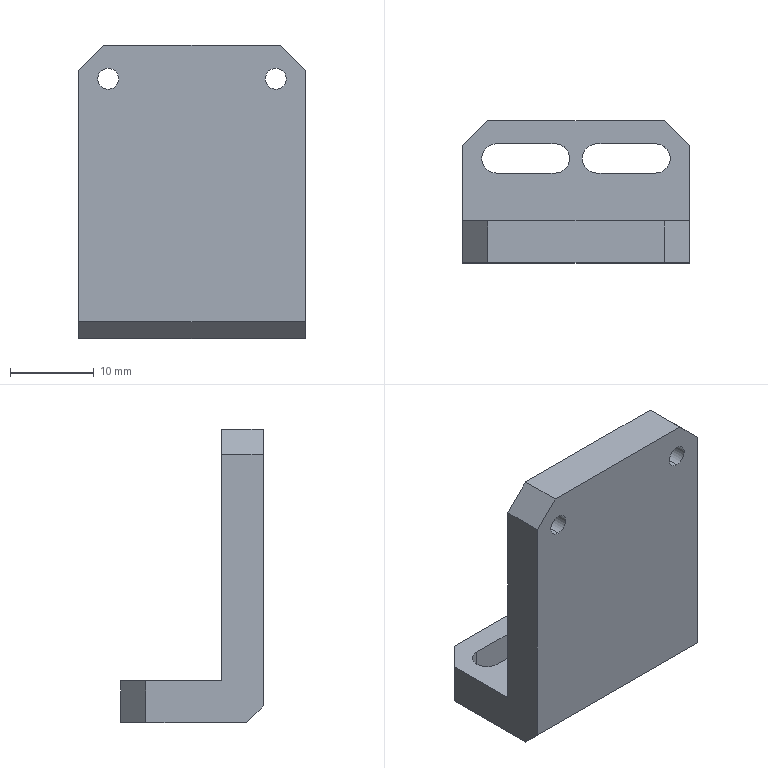Part | NX | features BREP 1 | 1 solid | 27 faces | box 27 x 17 x 35 mm | volume 5811 mm3 | plane 17 | cylinder 10 | commonest cylinder face diameters 3.5 x6 2.5 x4
STEP:
#1=CARTESIAN_POINT('',(-13.5,-3.,-17.5));
#2=VERTEX_POINT('',#1);
#3=CARTESIAN_POINT('',(-13.5,-5.,-15.5));
#4=VERTEX_POINT('',#3);
#5=CARTESIAN_POINT('',(-13.5,-5.,-15.5));
#6=DIRECTION('',(0.,-0.7071,0.7071));
#7=VECTOR('',#6,1000.);
#8=LINE('',#5,#7);
#9=EDGE_CURVE('',#2,#4,#8,.T.);
#10=ORIENTED_EDGE('',*,*,#9,.F.);
#11=CARTESIAN_POINT('',(13.5,-3.,-17.5));
#12=VERTEX_POINT('',#11);
#13=CARTESIAN_POINT('',(0.,-3.,-17.5));
#14=DIRECTION('',(-1.,0.,0.));
#15=VECTOR('',#14,1000.);
#16=LINE('',#13,#15);
#17=EDGE_CURVE('',#12,#2,#16,.T.);
#18=ORIENTED_EDGE('',*,*,#17,.F.);
#19=CARTESIAN_POINT('',(13.5,-5.,-15.5));
#20=VERTEX_POINT('',#19);
#21=CARTESIAN_POINT('',(13.5,-5.,-15.5));
#22=DIRECTION('',(0.,0.7071,-0.7071));
#23=VECTOR('',#22,1000.);
#24=LINE('',#21,#23);
#25=EDGE_CURVE('',#20,#12,#24,.T.);
#26=ORIENTED_EDGE('',*,*,#25,.F.);
#27=CARTESIAN_POINT('',(-13.5,-5.,-15.5));
#28=DIRECTION('',(1.,0.,0.));
#29=VECTOR('',#28,1000.);
#30=LINE('',#27,#29);
#31=EDGE_CURVE('',#4,#20,#30,.T.);
#32=ORIENTED_EDGE('',*,*,#31,.F.);
#33=EDGE_LOOP('',(#10,#18,#26,#32));
#34=FACE_BOUND('',#33,.T.);
#35=CARTESIAN_POINT('',(-13.5,-5.,-15.5));
#36=DIRECTION('',(0.,0.7071,0.7071));
#37=DIRECTION('',(1.,0.,0.));
#38=AXIS2_PLACEMENT_3D('',#35,#36,#37);
#39=PLANE('',#38);
#40=ADVANCED_FACE('',(#34),#39,.F.);
#41=CARTESIAN_POINT('',(-13.5,0.,14.5));
#42=VERTEX_POINT('',#41);
#43=CARTESIAN_POINT('',(-10.5,0.,17.5));
#44=VERTEX_POINT('',#43);
#45=CARTESIAN_POINT('',(-10.5,0.,17.5));
#46=DIRECTION('',(0.7071,0.,0.7071));
#47=VECTOR('',#46,1000.);
#48=LINE('',#45,#47);
#49=EDGE_CURVE('',#42,#44,#48,.T.);
#50=ORIENTED_EDGE('',*,*,#49,.F.);
#51=CARTESIAN_POINT('',(-13.5,-5.,14.5));
#52=VERTEX_POINT('',#51);
#53=CARTESIAN_POINT('',(-13.5,0.,14.5));
#54=DIRECTION('',(0.,1.,0.));
#55=VECTOR('',#54,1000.);
#56=LINE('',#53,#55);
#57=EDGE_CURVE('',#52,#42,#56,.T.);
#58=ORIENTED_EDGE('',*,*,#57,.F.);
#59=CARTESIAN_POINT('',(-10.5,-5.,17.5));
#60=VERTEX_POINT('',#59);
#61=CARTESIAN_POINT('',(-10.5,-5.,17.5));
#62=DIRECTION('',(-0.7071,0.,-0.7071));
#63=VECTOR('',#62,1000.);
#64=LINE('',#61,#63);
#65=EDGE_CURVE('',#60,#52,#64,.T.);
#66=ORIENTED_EDGE('',*,*,#65,.F.);
#67=CARTESIAN_POINT('',(-10.5,-5.,17.5));
#68=DIRECTION('',(0.,-1.,0.));
#69=VECTOR('',#68,1000.);
#70=LINE('',#67,#69);
#71=EDGE_CURVE('',#44,#60,#70,.T.);
#72=ORIENTED_EDGE('',*,*,#71,.F.);
#73=EDGE_LOOP('',(#50,#58,#66,#72));
#74=FACE_BOUND('',#73,.T.);
#75=CARTESIAN_POINT('',(-10.5,0.,17.5));
#76=DIRECTION('',(-0.7071,0.,0.7071));
#77=DIRECTION('',(0.,1.,0.));
#78=AXIS2_PLACEMENT_3D('',#75,#76,#77);
#79=PLANE('',#78);
#80=ADVANCED_FACE('',(#74),#79,.T.);
#81=CARTESIAN_POINT('',(13.5,-5.,14.5));
#82=VERTEX_POINT('',#81);
#83=CARTESIAN_POINT('',(10.5,-5.,17.5));
#84=VERTEX_POINT('',#83);
#85=CARTESIAN_POINT('',(10.5,-5.,17.5));
#86=DIRECTION('',(-0.7071,0.,0.7071));
#87=VECTOR('',#86,1000.);
#88=LINE('',#85,#87);
#89=EDGE_CURVE('',#82,#84,#88,.T.);
#90=ORIENTED_EDGE('',*,*,#89,.F.);
#91=CARTESIAN_POINT('',(13.5,0.,14.5));
#92=VERTEX_POINT('',#91);
#93=CARTESIAN_POINT('',(13.5,-5.,14.5));
#94=DIRECTION('',(0.,-1.,0.));
#95=VECTOR('',#94,1000.);
#96=LINE('',#93,#95);
#97=EDGE_CURVE('',#92,#82,#96,.T.);
#98=ORIENTED_EDGE('',*,*,#97,.F.);
#99=CARTESIAN_POINT('',(10.5,0.,17.5));
#100=VERTEX_POINT('',#99);
#101=CARTESIAN_POINT('',(10.5,0.,17.5));
#102=DIRECTION('',(0.7071,0.,-0.7071));
#103=VECTOR('',#102,1000.);
#104=LINE('',#101,#103);
#105=EDGE_CURVE('',#100,#92,#104,.T.);
#106=ORIENTED_EDGE('',*,*,#105,.F.);
#107=CARTESIAN_POINT('',(10.5,0.,17.5));
#108=DIRECTION('',(0.,1.,0.));
#109=VECTOR('',#108,1000.);
#110=LINE('',#107,#109);
#111=EDGE_CURVE('',#84,#100,#110,.T.);
#112=ORIENTED_EDGE('',*,*,#111,.F.);
#113=EDGE_LOOP('',(#90,#98,#106,#112));
#114=FACE_BOUND('',#113,.T.);
#115=CARTESIAN_POINT('',(10.5,0.,17.5));
#116=DIRECTION('',(0.7071,0.,0.7071));
#117=DIRECTION('',(0.,-1.,0.));
#118=AXIS2_PLACEMENT_3D('',#115,#116,#117);
#119=PLANE('',#118);
#120=ADVANCED_FACE('',(#114),#119,.T.);
#121=CARTESIAN_POINT('',(10.5,12.,-17.5));
#122=VERTEX_POINT('',#121);
#123=CARTESIAN_POINT('',(13.5,9.,-17.5));
#124=VERTEX_POINT('',#123);
#125=CARTESIAN_POINT('',(13.5,9.,-17.5));
#126=DIRECTION('',(0.7071,-0.7071,0.));
#127=VECTOR('',#126,1000.);
#128=LINE('',#125,#127);
#129=EDGE_CURVE('',#122,#124,#128,.T.);
#130=ORIENTED_EDGE('',*,*,#129,.F.);
#131=CARTESIAN_POINT('',(10.5,12.,-12.5));
#132=VERTEX_POINT('',#131);
#133=CARTESIAN_POINT('',(10.5,12.,-17.5));
#134=DIRECTION('',(0.,0.,-1.));
#135=VECTOR('',#134,1000.);
#136=LINE('',#133,#135);
#137=EDGE_CURVE('',#132,#122,#136,.T.);
#138=ORIENTED_EDGE('',*,*,#137,.F.);
#139=CARTESIAN_POINT('',(13.5,9.,-12.5));
#140=VERTEX_POINT('',#139);
#141=CARTESIAN_POINT('',(24.5,-2.,-12.5));
#142=DIRECTION('',(-0.7071,0.7071,0.));
#143=VECTOR('',#142,1000.);
#144=LINE('',#141,#143);
#145=EDGE_CURVE('',#140,#132,#144,.T.);
#146=ORIENTED_EDGE('',*,*,#145,.F.);
#147=CARTESIAN_POINT('',(13.5,9.,-12.5));
#148=DIRECTION('',(0.,0.,1.));
#149=VECTOR('',#148,1000.);
#150=LINE('',#147,#149);
#151=EDGE_CURVE('',#124,#140,#150,.T.);
#152=ORIENTED_EDGE('',*,*,#151,.F.);
#153=EDGE_LOOP('',(#130,#138,#146,#152));
#154=FACE_BOUND('',#153,.T.);
#155=CARTESIAN_POINT('',(13.5,9.,17.5));
#156=DIRECTION('',(0.7071,0.7071,0.));
#157=DIRECTION('',(0.,0.,-1.));
#158=AXIS2_PLACEMENT_3D('',#155,#156,#157);
#159=PLANE('',#158);
#160=ADVANCED_FACE('',(#154),#159,.T.);
#161=CARTESIAN_POINT('',(-10.5,12.,-12.5));
#162=VERTEX_POINT('',#161);
#163=CARTESIAN_POINT('',(-13.5,9.,-12.5));
#164=VERTEX_POINT('',#163);
#165=CARTESIAN_POINT('',(2.,24.5,-12.5));
#166=DIRECTION('',(-0.7071,-0.7071,0.));
#167=VECTOR('',#166,1000.);
#168=LINE('',#165,#167);
#169=EDGE_CURVE('',#162,#164,#168,.T.);
#170=ORIENTED_EDGE('',*,*,#169,.F.);
#171=CARTESIAN_POINT('',(-10.5,12.,-17.5));
#172=VERTEX_POINT('',#171);
#173=CARTESIAN_POINT('',(-10.5,12.,-12.5));
#174=DIRECTION('',(0.,0.,1.));
#175=VECTOR('',#174,1000.);
#176=LINE('',#173,#175);
#177=EDGE_CURVE('',#172,#162,#176,.T.);
#178=ORIENTED_EDGE('',*,*,#177,.F.);
#179=CARTESIAN_POINT('',(-13.5,9.,-17.5));
#180=VERTEX_POINT('',#179);
#181=CARTESIAN_POINT('',(-13.5,9.,-17.5));
#182=DIRECTION('',(0.7071,0.7071,0.));
#183=VECTOR('',#182,1000.);
#184=LINE('',#181,#183);
#185=EDGE_CURVE('',#180,#172,#184,.T.);
#186=ORIENTED_EDGE('',*,*,#185,.F.);
#187=CARTESIAN_POINT('',(-13.5,9.,-17.5));
#188=DIRECTION('',(0.,0.,-1.));
#189=VECTOR('',#188,1000.);
#190=LINE('',#187,#189);
#191=EDGE_CURVE('',#164,#180,#190,.T.);
#192=ORIENTED_EDGE('',*,*,#191,.F.);
#193=EDGE_LOOP('',(#170,#178,#186,#192));
#194=FACE_BOUND('',#193,.T.);
#195=CARTESIAN_POINT('',(-13.5,9.,17.5));
#196=DIRECTION('',(-0.7071,0.7071,0.));
#197=DIRECTION('',(0.,0.,1.));
#198=AXIS2_PLACEMENT_3D('',#195,#196,#197);
#199=PLANE('',#198);
#200=ADVANCED_FACE('',(#194),#199,.T.);
#201=CARTESIAN_POINT('',(9.5,9.25,-12.5));
#202=VERTEX_POINT('',#201);
#203=CARTESIAN_POINT('',(2.5,9.25,-12.5));
#204=VERTEX_POINT('',#203);
#205=CARTESIAN_POINT('',(9.5,9.25,-12.5));
#206=DIRECTION('',(-1.,0.,0.));
#207=VECTOR('',#206,1000.);
#208=LINE('',#205,#207);
#209=EDGE_CURVE('',#202,#204,#208,.T.);
#210=ORIENTED_EDGE('',*,*,#209,.T.);
#211=CARTESIAN_POINT('',(2.5,9.25,-17.5));
#212=VERTEX_POINT('',#211);
#213=CARTESIAN_POINT('',(2.5,9.25,-17.5));
#214=DIRECTION('',(0.,0.,1.));
#215=VECTOR('',#214,1000.);
#216=LINE('',#213,#215);
#217=EDGE_CURVE('',#212,#204,#216,.T.);
#218=ORIENTED_EDGE('',*,*,#217,.F.);
#219=CARTESIAN_POINT('',(9.5,9.25,-17.5));
#220=VERTEX_POINT('',#219);
#221=CARTESIAN_POINT('',(9.5,9.25,-17.5));
#222=DIRECTION('',(-1.,0.,0.));
#223=VECTOR('',#222,1000.);
#224=LINE('',#221,#223);
#225=EDGE_CURVE('',#220,#212,#224,.T.);
#226=ORIENTED_EDGE('',*,*,#225,.F.);
#227=CARTESIAN_POINT('',(9.5,9.25,-17.5));
#228=DIRECTION('',(0.,0.,1.));
#229=VECTOR('',#228,1000.);
#230=LINE('',#227,#229);
#231=EDGE_CURVE('',#220,#202,#230,.T.);
#232=ORIENTED_EDGE('',*,*,#231,.T.);
#233=EDGE_LOOP('',(#210,#218,#226,#232));
#234=FACE_BOUND('',#233,.T.);
#235=CARTESIAN_POINT('',(9.5,9.25,-17.5));
#236=DIRECTION('',(0.,1.,0.));
#237=DIRECTION('',(-1.,0.,0.));
#238=AXIS2_PLACEMENT_3D('',#235,#236,#237);
#239=PLANE('',#238);
#240=ADVANCED_FACE('',(#234),#239,.F.);
#241=CARTESIAN_POINT('',(2.5,5.75,-12.5));
#242=VERTEX_POINT('',#241);
#243=CARTESIAN_POINT('',(2.5,7.5,-12.5));
#244=DIRECTION('',(0.,0.,1.));
#245=DIRECTION('',(1.,0.,0.));
#246=AXIS2_PLACEMENT_3D('',#243,#244,#245);
#247=CIRCLE('',#246,1.75);
#248=EDGE_CURVE('',#204,#242,#247,.T.);
#249=ORIENTED_EDGE('',*,*,#248,.T.);
#250=CARTESIAN_POINT('',(2.5,5.75,-17.5));
#251=VERTEX_POINT('',#250);
#252=CARTESIAN_POINT('',(2.5,5.75,-17.5));
#253=DIRECTION('',(0.,0.,1.));
#254=VECTOR('',#253,1000.);
#255=LINE('',#252,#254);
#256=EDGE_CURVE('',#251,#242,#255,.T.);
#257=ORIENTED_EDGE('',*,*,#256,.F.);
#258=CARTESIAN_POINT('',(2.5,7.5,-17.5));
#259=DIRECTION('',(0.,0.,1.));
#260=DIRECTION('',(1.,0.,0.));
#261=AXIS2_PLACEMENT_3D('',#258,#259,#260);
#262=CIRCLE('',#261,1.75);
#263=EDGE_CURVE('',#212,#251,#262,.T.);
#264=ORIENTED_EDGE('',*,*,#263,.F.);
#265=ORIENTED_EDGE('',*,*,#217,.T.);
#266=EDGE_LOOP('',(#249,#257,#264,#265));
#267=FACE_BOUND('',#266,.T.);
#268=CARTESIAN_POINT('',(2.5,7.5,-17.5));
#269=DIRECTION('',(0.,0.,1.));
#270=DIRECTION('',(1.,0.,0.));
#271=AXIS2_PLACEMENT_3D('',#268,#269,#270);
#272=CYLINDRICAL_SURFACE('',#271,1.75);
#273=ADVANCED_FACE('',(#267),#272,.F.);
#274=CARTESIAN_POINT('',(9.5,5.75,-12.5));
#275=VERTEX_POINT('',#274);
#276=CARTESIAN_POINT('',(9.5,5.75,-12.5));
#277=DIRECTION('',(1.,0.,0.));
#278=VECTOR('',#277,1000.);
#279=LINE('',#276,#278);
#280=EDGE_CURVE('',#242,#275,#279,.T.);
#281=ORIENTED_EDGE('',*,*,#280,.T.);
#282=CARTESIAN_POINT('',(9.5,5.75,-17.5));
#283=VERTEX_POINT('',#282);
#284=CARTESIAN_POINT('',(9.5,5.75,-17.5));
#285=DIRECTION('',(0.,0.,1.));
#286=VECTOR('',#285,1000.);
#287=LINE('',#284,#286);
#288=EDGE_CURVE('',#283,#275,#287,.T.);
#289=ORIENTED_EDGE('',*,*,#288,.F.);
#290=CARTESIAN_POINT('',(9.5,5.75,-17.5));
#291=DIRECTION('',(1.,0.,0.));
#292=VECTOR('',#291,1000.);
#293=LINE('',#290,#292);
#294=EDGE_CURVE('',#251,#283,#293,.T.);
#295=ORIENTED_EDGE('',*,*,#294,.F.);
#296=ORIENTED_EDGE('',*,*,#256,.T.);
#297=EDGE_LOOP('',(#281,#289,#295,#296));
#298=FACE_BOUND('',#297,.T.);
#299=CARTESIAN_POINT('',(9.5,5.75,-17.5));
#300=DIRECTION('',(0.,-1.,0.));
#301=DIRECTION('',(1.,0.,0.));
#302=AXIS2_PLACEMENT_3D('',#299,#300,#301);
#303=PLANE('',#302);
#304=ADVANCED_FACE('',(#298),#303,.F.);
#305=CARTESIAN_POINT('',(11.25,7.5,-17.5));
#306=VERTEX_POINT('',#305);
#307=CARTESIAN_POINT('',(11.25,7.5,-12.5));
#308=VERTEX_POINT('',#307);
#309=CARTESIAN_POINT('',(11.25,7.5,-17.5));
#310=DIRECTION('',(0.,0.,1.));
#311=VECTOR('',#310,1000.);
#312=LINE('',#309,#311);
#313=EDGE_CURVE('',#306,#308,#312,.T.);
#314=ORIENTED_EDGE('',*,*,#313,.F.);
#315=CARTESIAN_POINT('',(9.5,7.5,-17.5));
#316=DIRECTION('',(0.,0.,1.));
#317=DIRECTION('',(1.,0.,0.));
#318=AXIS2_PLACEMENT_3D('',#315,#316,#317);
#319=CIRCLE('',#318,1.75);
#320=EDGE_CURVE('',#283,#306,#319,.T.);
#321=ORIENTED_EDGE('',*,*,#320,.F.);
#322=ORIENTED_EDGE('',*,*,#288,.T.);
#323=CARTESIAN_POINT('',(9.5,7.5,-12.5));
#324=DIRECTION('',(0.,0.,1.));
#325=DIRECTION('',(1.,0.,0.));
#326=AXIS2_PLACEMENT_3D('',#323,#324,#325);
#327=CIRCLE('',#326,1.75);
#328=EDGE_CURVE('',#275,#308,#327,.T.);
#329=ORIENTED_EDGE('',*,*,#328,.T.);
#330=EDGE_LOOP('',(#314,#321,#322,#329));
#331=FACE_BOUND('',#330,.T.);
#332=CARTESIAN_POINT('',(9.5,7.5,-17.5));
#333=DIRECTION('',(0.,0.,1.));
#334=DIRECTION('',(1.,0.,0.));
#335=AXIS2_PLACEMENT_3D('',#332,#333,#334);
#336=CYLINDRICAL_SURFACE('',#335,1.75);
#337=ADVANCED_FACE('',(#331),#336,.F.);
#338=CARTESIAN_POINT('',(-9.5,5.75,-12.5));
#339=VERTEX_POINT('',#338);
#340=CARTESIAN_POINT('',(-2.5,5.75,-12.5));
#341=VERTEX_POINT('',#340);
#342=CARTESIAN_POINT('',(-9.5,5.75,-12.5));
#343=DIRECTION('',(1.,0.,0.));
#344=VECTOR('',#343,1000.);
#345=LINE('',#342,#344);
#346=EDGE_CURVE('',#339,#341,#345,.T.);
#347=ORIENTED_EDGE('',*,*,#346,.T.);
#348=CARTESIAN_POINT('',(-2.5,5.75,-17.5));
#349=VERTEX_POINT('',#348);
#350=CARTESIAN_POINT('',(-2.5,5.75,-17.5));
#351=DIRECTION('',(0.,0.,1.));
#352=VECTOR('',#351,1000.);
#353=LINE('',#350,#352);
#354=EDGE_CURVE('',#349,#341,#353,.T.);
#355=ORIENTED_EDGE('',*,*,#354,.F.);
#356=CARTESIAN_POINT('',(-9.5,5.75,-17.5));
#357=VERTEX_POINT('',#356);
#358=CARTESIAN_POINT('',(-9.5,5.75,-17.5));
#359=DIRECTION('',(1.,0.,0.));
#360=VECTOR('',#359,1000.);
#361=LINE('',#358,#360);
#362=EDGE_CURVE('',#357,#349,#361,.T.);
#363=ORIENTED_EDGE('',*,*,#362,.F.);
#364=CARTESIAN_POINT('',(-9.5,5.75,-17.5));
#365=DIRECTION('',(0.,0.,1.));
#366=VECTOR('',#365,1000.);
#367=LINE('',#364,#366);
#368=EDGE_CURVE('',#357,#339,#367,.T.);
#369=ORIENTED_EDGE('',*,*,#368,.T.);
#370=EDGE_LOOP('',(#347,#355,#363,#369));
#371=FACE_BOUND('',#370,.T.);
#372=CARTESIAN_POINT('',(-9.5,5.75,-17.5));
#373=DIRECTION('',(0.,-1.,0.));
#374=DIRECTION('',(1.,0.,0.));
#375=AXIS2_PLACEMENT_3D('',#372,#373,#374);
#376=PLANE('',#375);
#377=ADVANCED_FACE('',(#371),#376,.F.);
#378=CARTESIAN_POINT('',(-0.75,7.5,-17.5));
#379=VERTEX_POINT('',#378);
#380=CARTESIAN_POINT('',(-0.75,7.5,-12.5));
#381=VERTEX_POINT('',#380);
#382=CARTESIAN_POINT('',(-0.75,7.5,-17.5));
#383=DIRECTION('',(0.,0.,1.));
#384=VECTOR('',#383,1000.);
#385=LINE('',#382,#384);
#386=EDGE_CURVE('',#379,#381,#385,.T.);
#387=ORIENTED_EDGE('',*,*,#386,.F.);
#388=CARTESIAN_POINT('',(-2.5,7.5,-17.5));
#389=DIRECTION('',(0.,0.,1.));
#390=DIRECTION('',(1.,0.,0.));
#391=AXIS2_PLACEMENT_3D('',#388,#389,#390);
#392=CIRCLE('',#391,1.75);
#393=EDGE_CURVE('',#349,#379,#392,.T.);
#394=ORIENTED_EDGE('',*,*,#393,.F.);
#395=ORIENTED_EDGE('',*,*,#354,.T.);
#396=CARTESIAN_POINT('',(-2.5,7.5,-12.5));
#397=DIRECTION('',(0.,0.,1.));
#398=DIRECTION('',(1.,0.,0.));
#399=AXIS2_PLACEMENT_3D('',#396,#397,#398);
#400=CIRCLE('',#399,1.75);
#401=EDGE_CURVE('',#341,#381,#400,.T.);
#402=ORIENTED_EDGE('',*,*,#401,.T.);
#403=EDGE_LOOP('',(#387,#394,#395,#402));
#404=FACE_BOUND('',#403,.T.);
#405=CARTESIAN_POINT('',(-2.5,7.5,-17.5));
#406=DIRECTION('',(0.,0.,1.));
#407=DIRECTION('',(1.,0.,0.));
#408=AXIS2_PLACEMENT_3D('',#405,#406,#407);
#409=CYLINDRICAL_SURFACE('',#408,1.75);
#410=ADVANCED_FACE('',(#404),#409,.F.);
#411=CARTESIAN_POINT('',(-2.5,9.25,-12.5));
#412=VERTEX_POINT('',#411);
#413=CARTESIAN_POINT('',(-9.5,9.25,-12.5));
#414=VERTEX_POINT('',#413);
#415=CARTESIAN_POINT('',(-9.5,9.25,-12.5));
#416=DIRECTION('',(-1.,0.,0.));
#417=VECTOR('',#416,1000.);
#418=LINE('',#415,#417);
#419=EDGE_CURVE('',#412,#414,#418,.T.);
#420=ORIENTED_EDGE('',*,*,#419,.T.);
#421=CARTESIAN_POINT('',(-9.5,9.25,-17.5));
#422=VERTEX_POINT('',#421);
#423=CARTESIAN_POINT('',(-9.5,9.25,-17.5));
#424=DIRECTION('',(0.,0.,1.));
#425=VECTOR('',#424,1000.);
#426=LINE('',#423,#425);
#427=EDGE_CURVE('',#422,#414,#426,.T.);
#428=ORIENTED_EDGE('',*,*,#427,.F.);
#429=CARTESIAN_POINT('',(-2.5,9.25,-17.5));
#430=VERTEX_POINT('',#429);
#431=CARTESIAN_POINT('',(-9.5,9.25,-17.5));
#432=DIRECTION('',(-1.,0.,0.));
#433=VECTOR('',#432,1000.);
#434=LINE('',#431,#433);
#435=EDGE_CURVE('',#430,#422,#434,.T.);
#436=ORIENTED_EDGE('',*,*,#435,.F.);
#437=CARTESIAN_POINT('',(-2.5,9.25,-17.5));
#438=DIRECTION('',(0.,0.,1.));
#439=VECTOR('',#438,1000.);
#440=LINE('',#437,#439);
#441=EDGE_CURVE('',#430,#412,#440,.T.);
#442=ORIENTED_EDGE('',*,*,#441,.T.);
#443=EDGE_LOOP('',(#420,#428,#436,#442));
#444=FACE_BOUND('',#443,.T.);
#445=CARTESIAN_POINT('',(-9.5,9.25,-17.5));
#446=DIRECTION('',(0.,1.,0.));
#447=DIRECTION('',(-1.,0.,0.));
#448=AXIS2_PLACEMENT_3D('',#445,#446,#447);
#449=PLANE('',#448);
#450=ADVANCED_FACE('',(#444),#449,.F.);
#451=CARTESIAN_POINT('',(-9.5,7.5,-12.5));
#452=DIRECTION('',(0.,0.,1.));
#453=DIRECTION('',(1.,0.,0.));
#454=AXIS2_PLACEMENT_3D('',#451,#452,#453);
#455=CIRCLE('',#454,1.75);
#456=EDGE_CURVE('',#414,#339,#455,.T.);
#457=ORIENTED_EDGE('',*,*,#456,.T.);
#458=ORIENTED_EDGE('',*,*,#368,.F.);
#459=CARTESIAN_POINT('',(-9.5,7.5,-17.5));
#460=DIRECTION('',(0.,0.,1.));
#461=DIRECTION('',(1.,0.,0.));
#462=AXIS2_PLACEMENT_3D('',#459,#460,#461);
#463=CIRCLE('',#462,1.75);
#464=EDGE_CURVE('',#422,#357,#463,.T.);
#465=ORIENTED_EDGE('',*,*,#464,.F.);
#466=ORIENTED_EDGE('',*,*,#427,.T.);
#467=EDGE_LOOP('',(#457,#458,#465,#466));
#468=FACE_BOUND('',#467,.T.);
#469=CARTESIAN_POINT('',(-9.5,7.5,-17.5));
#470=DIRECTION('',(0.,0.,1.));
#471=DIRECTION('',(1.,0.,0.));
#472=AXIS2_PLACEMENT_3D('',#469,#470,#471);
#473=CYLINDRICAL_SURFACE('',#472,1.75);
#474=ADVANCED_FACE('',(#468),#473,.F.);
#475=CARTESIAN_POINT('',(26.5,12.,-12.5));
#476=DIRECTION('',(-1.,0.,0.));
#477=VECTOR('',#476,1000.);
#478=LINE('',#475,#477);
#479=EDGE_CURVE('',#132,#162,#478,.T.);
#480=ORIENTED_EDGE('',*,*,#479,.T.);
#481=ORIENTED_EDGE('',*,*,#169,.T.);
#482=CARTESIAN_POINT('',(-13.5,0.,-12.5));
#483=VERTEX_POINT('',#482);
#484=CARTESIAN_POINT('',(-13.5,0.,-12.5));
#485=DIRECTION('',(0.,1.,0.));
#486=VECTOR('',#485,1000.);
#487=LINE('',#484,#486);
#488=EDGE_CURVE('',#483,#164,#487,.T.);
#489=ORIENTED_EDGE('',*,*,#488,.F.);
#490=CARTESIAN_POINT('',(13.5,0.,-12.5));
#491=VERTEX_POINT('',#490);
#492=CARTESIAN_POINT('',(26.5,0.,-12.5));
#493=DIRECTION('',(-1.,0.,0.));
#494=VECTOR('',#493,1000.);
#495=LINE('',#492,#494);
#496=EDGE_CURVE('',#491,#483,#495,.T.);
#497=ORIENTED_EDGE('',*,*,#496,.F.);
#498=CARTESIAN_POINT('',(13.5,0.,-12.5));
#499=DIRECTION('',(0.,-1.,0.));
#500=VECTOR('',#499,1000.);
#501=LINE('',#498,#500);
#502=EDGE_CURVE('',#140,#491,#501,.T.);
#503=ORIENTED_EDGE('',*,*,#502,.F.);
#504=ORIENTED_EDGE('',*,*,#145,.T.);
#505=EDGE_LOOP('',(#480,#481,#489,#497,#503,#504));
#506=FACE_BOUND('',#505,.T.);
#507=ORIENTED_EDGE('',*,*,#456,.F.);
#508=ORIENTED_EDGE('',*,*,#419,.F.);
#509=CARTESIAN_POINT('',(-2.5,7.5,-12.5));
#510=DIRECTION('',(0.,0.,1.));
#511=DIRECTION('',(1.,0.,0.));
#512=AXIS2_PLACEMENT_3D('',#509,#510,#511);
#513=CIRCLE('',#512,1.75);
#514=EDGE_CURVE('',#381,#412,#513,.T.);
#515=ORIENTED_EDGE('',*,*,#514,.F.);
#516=ORIENTED_EDGE('',*,*,#401,.F.);
#517=ORIENTED_EDGE('',*,*,#346,.F.);
#518=EDGE_LOOP('',(#507,#508,#515,#516,#517));
#519=FACE_BOUND('',#518,.T.);
#520=ORIENTED_EDGE('',*,*,#328,.F.);
#521=ORIENTED_EDGE('',*,*,#280,.F.);
#522=ORIENTED_EDGE('',*,*,#248,.F.);
#523=ORIENTED_EDGE('',*,*,#209,.F.);
#524=CARTESIAN_POINT('',(9.5,7.5,-12.5));
#525=DIRECTION('',(0.,0.,1.));
#526=DIRECTION('',(1.,0.,0.));
#527=AXIS2_PLACEMENT_3D('',#524,#525,#526);
#528=CIRCLE('',#527,1.75);
#529=EDGE_CURVE('',#308,#202,#528,.T.);
#530=ORIENTED_EDGE('',*,*,#529,.F.);
#531=EDGE_LOOP('',(#520,#521,#522,#523,#530));
#532=FACE_BOUND('',#531,.T.);
#533=CARTESIAN_POINT('',(26.5,0.,-12.5));
#534=DIRECTION('',(0.,0.,1.));
#535=DIRECTION('',(1.,0.,0.));
#536=AXIS2_PLACEMENT_3D('',#533,#534,#535);
#537=PLANE('',#536);
#538=ADVANCED_FACE('',(#506,#519,#532),#537,.T.);
#539=CARTESIAN_POINT('',(26.5,12.,-17.5));
#540=DIRECTION('',(-1.,0.,0.));
#541=VECTOR('',#540,1000.);
#542=LINE('',#539,#541);
#543=EDGE_CURVE('',#122,#172,#542,.T.);
#544=ORIENTED_EDGE('',*,*,#543,.T.);
#545=ORIENTED_EDGE('',*,*,#177,.T.);
#546=ORIENTED_EDGE('',*,*,#479,.F.);
#547=ORIENTED_EDGE('',*,*,#137,.T.);
#548=EDGE_LOOP('',(#544,#545,#546,#547));
#549=FACE_BOUND('',#548,.T.);
#550=CARTESIAN_POINT('',(26.5,12.,-17.5));
#551=DIRECTION('',(0.,1.,0.));
#552=DIRECTION('',(0.,0.,1.));
#553=AXIS2_PLACEMENT_3D('',#550,#551,#552);
#554=PLANE('',#553);
#555=ADVANCED_FACE('',(#549),#554,.T.);
#556=CARTESIAN_POINT('',(-10.,0.,12.25));
#557=VERTEX_POINT('',#556);
#558=CARTESIAN_POINT('',(-10.,-5.,12.25));
#559=VERTEX_POINT('',#558);
#560=CARTESIAN_POINT('',(-10.,0.,12.25));
#561=DIRECTION('',(0.,1.,0.));
#562=VECTOR('',#561,1000.);
#563=LINE('',#560,#562);
#564=EDGE_CURVE('',#557,#559,#563,.F.);
#565=ORIENTED_EDGE('',*,*,#564,.T.);
#566=CARTESIAN_POINT('',(-10.,-5.,14.75));
#567=VERTEX_POINT('',#566);
#568=CARTESIAN_POINT('',(-10.,-5.,13.5));
#569=DIRECTION('',(0.,1.,0.));
#570=DIRECTION('',(0.,0.,1.));
#571=AXIS2_PLACEMENT_3D('',#568,#569,#570);
#572=CIRCLE('',#571,1.25);
#573=EDGE_CURVE('',#567,#559,#572,.T.);
#574=ORIENTED_EDGE('',*,*,#573,.F.);
#575=CARTESIAN_POINT('',(-10.,0.,14.75));
#576=VERTEX_POINT('',#575);
#577=CARTESIAN_POINT('',(-10.,0.,14.75));
#578=DIRECTION('',(0.,1.,0.));
#579=VECTOR('',#578,1000.);
#580=LINE('',#577,#579);
#581=EDGE_CURVE('',#576,#567,#580,.F.);
#582=ORIENTED_EDGE('',*,*,#581,.F.);
#583=CARTESIAN_POINT('',(-10.,0.,13.5));
#584=DIRECTION('',(0.,1.,0.));
#585=DIRECTION('',(0.,0.,1.));
#586=AXIS2_PLACEMENT_3D('',#583,#584,#585);
#587=CIRCLE('',#586,1.25);
#588=EDGE_CURVE('',#576,#557,#587,.T.);
#589=ORIENTED_EDGE('',*,*,#588,.T.);
#590=EDGE_LOOP('',(#565,#574,#582,#589));
#591=FACE_BOUND('',#590,.T.);
#592=CARTESIAN_POINT('',(-10.,0.,13.5));
#593=DIRECTION('',(0.,1.,0.));
#594=DIRECTION('',(0.,0.,1.));
#595=AXIS2_PLACEMENT_3D('',#592,#593,#594);
#596=CYLINDRICAL_SURFACE('',#595,1.25);
#597=ADVANCED_FACE('',(#591),#596,.F.);
#598=CARTESIAN_POINT('',(10.,0.,12.25));
#599=VERTEX_POINT('',#598);
#600=CARTESIAN_POINT('',(10.,-5.,12.25));
#601=VERTEX_POINT('',#600);
#602=CARTESIAN_POINT('',(10.,0.,12.25));
#603=DIRECTION('',(0.,1.,0.));
#604=VECTOR('',#603,1000.);
#605=LINE('',#602,#604);
#606=EDGE_CURVE('',#599,#601,#605,.F.);
#607=ORIENTED_EDGE('',*,*,#606,.T.);
#608=CARTESIAN_POINT('',(10.,-5.,14.75));
#609=VERTEX_POINT('',#608);
#610=CARTESIAN_POINT('',(10.,-5.,13.5));
#611=DIRECTION('',(0.,1.,0.));
#612=DIRECTION('',(0.,0.,1.));
#613=AXIS2_PLACEMENT_3D('',#610,#611,#612);
#614=CIRCLE('',#613,1.25);
#615=EDGE_CURVE('',#609,#601,#614,.T.);
#616=ORIENTED_EDGE('',*,*,#615,.F.);
#617=CARTESIAN_POINT('',(10.,0.,14.75));
#618=VERTEX_POINT('',#617);
#619=CARTESIAN_POINT('',(10.,0.,14.75));
#620=DIRECTION('',(0.,1.,0.));
#621=VECTOR('',#620,1000.);
#622=LINE('',#619,#621);
#623=EDGE_CURVE('',#618,#609,#622,.F.);
#624=ORIENTED_EDGE('',*,*,#623,.F.);
#625=CARTESIAN_POINT('',(10.,0.,13.5));
#626=DIRECTION('',(0.,1.,0.));
#627=DIRECTION('',(0.,0.,1.));
#628=AXIS2_PLACEMENT_3D('',#625,#626,#627);
#629=CIRCLE('',#628,1.25);
#630=EDGE_CURVE('',#618,#599,#629,.T.);
#631=ORIENTED_EDGE('',*,*,#630,.T.);
#632=EDGE_LOOP('',(#607,#616,#624,#631));
#633=FACE_BOUND('',#632,.T.);
#634=CARTESIAN_POINT('',(10.,0.,13.5));
#635=DIRECTION('',(0.,1.,0.));
#636=DIRECTION('',(0.,0.,1.));
#637=AXIS2_PLACEMENT_3D('',#634,#635,#636);
#638=CYLINDRICAL_SURFACE('',#637,1.25);
#639=ADVANCED_FACE('',(#633),#638,.F.);
#640=CARTESIAN_POINT('',(13.5,-5.,-17.5));
#641=DIRECTION('',(0.,1.,0.));
#642=VECTOR('',#641,1000.);
#643=LINE('',#640,#642);
#644=EDGE_CURVE('',#12,#124,#643,.T.);
#645=ORIENTED_EDGE('',*,*,#644,.F.);
#646=ORIENTED_EDGE('',*,*,#17,.T.);
#647=CARTESIAN_POINT('',(-13.5,0.,-17.5));
#648=DIRECTION('',(0.,-1.,0.));
#649=VECTOR('',#648,1000.);
#650=LINE('',#647,#649);
#651=EDGE_CURVE('',#180,#2,#650,.T.);
#652=ORIENTED_EDGE('',*,*,#651,.F.);
#653=ORIENTED_EDGE('',*,*,#185,.T.);
#654=ORIENTED_EDGE('',*,*,#543,.F.);
#655=ORIENTED_EDGE('',*,*,#129,.T.);
#656=EDGE_LOOP('',(#645,#646,#652,#653,#654,#655));
#657=FACE_BOUND('',#656,.T.);
#658=ORIENTED_EDGE('',*,*,#435,.T.);
#659=ORIENTED_EDGE('',*,*,#464,.T.);
#660=ORIENTED_EDGE('',*,*,#362,.T.);
#661=ORIENTED_EDGE('',*,*,#393,.T.);
#662=CARTESIAN_POINT('',(-2.5,7.5,-17.5));
#663=DIRECTION('',(0.,0.,1.));
#664=DIRECTION('',(1.,0.,0.));
#665=AXIS2_PLACEMENT_3D('',#662,#663,#664);
#666=CIRCLE('',#665,1.75);
#667=EDGE_CURVE('',#379,#430,#666,.T.);
#668=ORIENTED_EDGE('',*,*,#667,.T.);
#669=EDGE_LOOP('',(#658,#659,#660,#661,#668));
#670=FACE_BOUND('',#669,.T.);
#671=ORIENTED_EDGE('',*,*,#294,.T.);
#672=ORIENTED_EDGE('',*,*,#320,.T.);
#673=CARTESIAN_POINT('',(9.5,7.5,-17.5));
#674=DIRECTION('',(0.,0.,1.));
#675=DIRECTION('',(1.,0.,0.));
#676=AXIS2_PLACEMENT_3D('',#673,#674,#675);
#677=CIRCLE('',#676,1.75);
#678=EDGE_CURVE('',#306,#220,#677,.T.);
#679=ORIENTED_EDGE('',*,*,#678,.T.);
#680=ORIENTED_EDGE('',*,*,#225,.T.);
#681=ORIENTED_EDGE('',*,*,#263,.T.);
#682=EDGE_LOOP('',(#671,#672,#679,#680,#681));
#683=FACE_BOUND('',#682,.T.);
#684=CARTESIAN_POINT('',(0.,0.,-17.5));
#685=DIRECTION('',(0.,0.,1.));
#686=DIRECTION('',(1.,0.,0.));
#687=AXIS2_PLACEMENT_3D('',#684,#685,#686);
#688=PLANE('',#687);
#689=ADVANCED_FACE('',(#657,#670,#683),#688,.F.);
#690=CARTESIAN_POINT('',(-13.5,-5.,17.5));
#691=DIRECTION('',(1.,0.,0.));
#692=VECTOR('',#691,1000.);
#693=LINE('',#690,#692);
#694=EDGE_CURVE('',#60,#84,#693,.T.);
#695=ORIENTED_EDGE('',*,*,#694,.T.);
#696=ORIENTED_EDGE('',*,*,#111,.T.);
#697=CARTESIAN_POINT('',(13.5,0.,17.5));
#698=DIRECTION('',(-1.,0.,0.));
#699=VECTOR('',#698,1000.);
#700=LINE('',#697,#699);
#701=EDGE_CURVE('',#100,#44,#700,.T.);
#702=ORIENTED_EDGE('',*,*,#701,.T.);
#703=ORIENTED_EDGE('',*,*,#71,.T.);
#704=EDGE_LOOP('',(#695,#696,#702,#703));
#705=FACE_BOUND('',#704,.T.);
#706=CARTESIAN_POINT('',(0.,0.,17.5));
#707=DIRECTION('',(0.,0.,1.));
#708=DIRECTION('',(1.,0.,0.));
#709=AXIS2_PLACEMENT_3D('',#706,#707,#708);
#710=PLANE('',#709);
#711=ADVANCED_FACE('',(#705),#710,.T.);
#712=CARTESIAN_POINT('',(13.5,-5.,17.5));
#713=DIRECTION('',(0.,0.,-1.));
#714=VECTOR('',#713,1000.);
#715=LINE('',#712,#714);
#716=EDGE_CURVE('',#82,#20,#715,.T.);
#717=ORIENTED_EDGE('',*,*,#716,.T.);
#718=ORIENTED_EDGE('',*,*,#25,.T.);
#719=ORIENTED_EDGE('',*,*,#644,.T.);
#720=ORIENTED_EDGE('',*,*,#151,.T.);
#721=ORIENTED_EDGE('',*,*,#502,.T.);
#722=CARTESIAN_POINT('',(13.5,0.,17.5));
#723=DIRECTION('',(0.,0.,-1.));
#724=VECTOR('',#723,1000.);
#725=LINE('',#722,#724);
#726=EDGE_CURVE('',#92,#491,#725,.T.);
#727=ORIENTED_EDGE('',*,*,#726,.F.);
#728=ORIENTED_EDGE('',*,*,#97,.T.);
#729=EDGE_LOOP('',(#717,#718,#719,#720,#721,#727,#728));
#730=FACE_BOUND('',#729,.T.);
#731=CARTESIAN_POINT('',(13.5,-5.,17.5));
#732=DIRECTION('',(-1.,0.,0.));
#733=DIRECTION('',(0.,0.,1.));
#734=AXIS2_PLACEMENT_3D('',#731,#732,#733);
#735=PLANE('',#734);
#736=ADVANCED_FACE('',(#730),#735,.F.);
#737=CARTESIAN_POINT('',(-13.5,-5.,17.5));
#738=DIRECTION('',(0.,0.,-1.));
#739=VECTOR('',#738,1000.);
#740=LINE('',#737,#739);
#741=EDGE_CURVE('',#52,#4,#740,.T.);
#742=ORIENTED_EDGE('',*,*,#741,.T.);
#743=ORIENTED_EDGE('',*,*,#31,.T.);
#744=ORIENTED_EDGE('',*,*,#716,.F.);
#745=ORIENTED_EDGE('',*,*,#89,.T.);
#746=ORIENTED_EDGE('',*,*,#694,.F.);
#747=ORIENTED_EDGE('',*,*,#65,.T.);
#748=EDGE_LOOP('',(#742,#743,#744,#745,#746,#747));
#749=FACE_BOUND('',#748,.T.);
#750=ORIENTED_EDGE('',*,*,#615,.T.);
#751=CARTESIAN_POINT('',(10.,-5.,13.5));
#752=DIRECTION('',(0.,1.,0.));
#753=DIRECTION('',(0.,0.,1.));
#754=AXIS2_PLACEMENT_3D('',#751,#752,#753);
#755=CIRCLE('',#754,1.25);
#756=EDGE_CURVE('',#601,#609,#755,.T.);
#757=ORIENTED_EDGE('',*,*,#756,.T.);
#758=EDGE_LOOP('',(#750,#757));
#759=FACE_BOUND('',#758,.T.);
#760=ORIENTED_EDGE('',*,*,#573,.T.);
#761=CARTESIAN_POINT('',(-10.,-5.,13.5));
#762=DIRECTION('',(0.,1.,0.));
#763=DIRECTION('',(0.,0.,1.));
#764=AXIS2_PLACEMENT_3D('',#761,#762,#763);
#765=CIRCLE('',#764,1.25);
#766=EDGE_CURVE('',#559,#567,#765,.T.);
#767=ORIENTED_EDGE('',*,*,#766,.T.);
#768=EDGE_LOOP('',(#760,#767));
#769=FACE_BOUND('',#768,.T.);
#770=CARTESIAN_POINT('',(-13.5,-5.,17.5));
#771=DIRECTION('',(0.,1.,0.));
#772=DIRECTION('',(0.,0.,1.));
#773=AXIS2_PLACEMENT_3D('',#770,#771,#772);
#774=PLANE('',#773);
#775=ADVANCED_FACE('',(#749,#759,#769),#774,.F.);
#776=ORIENTED_EDGE('',*,*,#651,.T.);
#777=ORIENTED_EDGE('',*,*,#9,.T.);
#778=ORIENTED_EDGE('',*,*,#741,.F.);
#779=ORIENTED_EDGE('',*,*,#57,.T.);
#780=CARTESIAN_POINT('',(-13.5,0.,17.5));
#781=DIRECTION('',(0.,0.,-1.));
#782=VECTOR('',#781,1000.);
#783=LINE('',#780,#782);
#784=EDGE_CURVE('',#42,#483,#783,.T.);
#785=ORIENTED_EDGE('',*,*,#784,.T.);
#786=ORIENTED_EDGE('',*,*,#488,.T.);
#787=ORIENTED_EDGE('',*,*,#191,.T.);
#788=EDGE_LOOP('',(#776,#777,#778,#779,#785,#786,#787));
#789=FACE_BOUND('',#788,.T.);
#790=CARTESIAN_POINT('',(-13.5,0.,17.5));
#791=DIRECTION('',(1.,0.,0.));
#792=DIRECTION('',(0.,0.,-1.));
#793=AXIS2_PLACEMENT_3D('',#790,#791,#792);
#794=PLANE('',#793);
#795=ADVANCED_FACE('',(#789),#794,.F.);
#796=ORIENTED_EDGE('',*,*,#701,.F.);
#797=ORIENTED_EDGE('',*,*,#105,.T.);
#798=ORIENTED_EDGE('',*,*,#726,.T.);
#799=ORIENTED_EDGE('',*,*,#496,.T.);
#800=ORIENTED_EDGE('',*,*,#784,.F.);
#801=ORIENTED_EDGE('',*,*,#49,.T.);
#802=EDGE_LOOP('',(#796,#797,#798,#799,#800,#801));
#803=FACE_BOUND('',#802,.T.);
#804=ORIENTED_EDGE('',*,*,#630,.F.);
#805=CARTESIAN_POINT('',(10.,0.,13.5));
#806=DIRECTION('',(0.,1.,0.));
#807=DIRECTION('',(0.,0.,1.));
#808=AXIS2_PLACEMENT_3D('',#805,#806,#807);
#809=CIRCLE('',#808,1.25);
#810=EDGE_CURVE('',#599,#618,#809,.T.);
#811=ORIENTED_EDGE('',*,*,#810,.F.);
#812=EDGE_LOOP('',(#804,#811));
#813=FACE_BOUND('',#812,.T.);
#814=ORIENTED_EDGE('',*,*,#588,.F.);
#815=CARTESIAN_POINT('',(-10.,0.,13.5));
#816=DIRECTION('',(0.,1.,0.));
#817=DIRECTION('',(0.,0.,1.));
#818=AXIS2_PLACEMENT_3D('',#815,#816,#817);
#819=CIRCLE('',#818,1.25);
#820=EDGE_CURVE('',#557,#576,#819,.T.);
#821=ORIENTED_EDGE('',*,*,#820,.F.);
#822=EDGE_LOOP('',(#814,#821));
#823=FACE_BOUND('',#822,.T.);
#824=CARTESIAN_POINT('',(13.5,0.,17.5));
#825=DIRECTION('',(0.,-1.,0.));
#826=DIRECTION('',(0.,0.,-1.));
#827=AXIS2_PLACEMENT_3D('',#824,#825,#826);
#828=PLANE('',#827);
#829=ADVANCED_FACE('',(#803,#813,#823),#828,.F.);
#830=ORIENTED_EDGE('',*,*,#756,.F.);
#831=ORIENTED_EDGE('',*,*,#606,.F.);
#832=ORIENTED_EDGE('',*,*,#810,.T.);
#833=ORIENTED_EDGE('',*,*,#623,.T.);
#834=EDGE_LOOP('',(#830,#831,#832,#833));
#835=FACE_BOUND('',#834,.T.);
#836=CARTESIAN_POINT('',(10.,0.,13.5));
#837=DIRECTION('',(0.,1.,0.));
#838=DIRECTION('',(0.,0.,1.));
#839=AXIS2_PLACEMENT_3D('',#836,#837,#838);
#840=CYLINDRICAL_SURFACE('',#839,1.25);
#841=ADVANCED_FACE('',(#835),#840,.F.);
#842=ORIENTED_EDGE('',*,*,#766,.F.);
#843=ORIENTED_EDGE('',*,*,#564,.F.);
#844=ORIENTED_EDGE('',*,*,#820,.T.);
#845=ORIENTED_EDGE('',*,*,#581,.T.);
#846=EDGE_LOOP('',(#842,#843,#844,#845));
#847=FACE_BOUND('',#846,.T.);
#848=CARTESIAN_POINT('',(-10.,0.,13.5));
#849=DIRECTION('',(0.,1.,0.));
#850=DIRECTION('',(0.,0.,1.));
#851=AXIS2_PLACEMENT_3D('',#848,#849,#850);
#852=CYLINDRICAL_SURFACE('',#851,1.25);
#853=ADVANCED_FACE('',(#847),#852,.F.);
#854=ORIENTED_EDGE('',*,*,#667,.F.);
#855=ORIENTED_EDGE('',*,*,#386,.T.);
#856=ORIENTED_EDGE('',*,*,#514,.T.);
#857=ORIENTED_EDGE('',*,*,#441,.F.);
#858=EDGE_LOOP('',(#854,#855,#856,#857));
#859=FACE_BOUND('',#858,.T.);
#860=CARTESIAN_POINT('',(-2.5,7.5,-17.5));
#861=DIRECTION('',(0.,0.,1.));
#862=DIRECTION('',(1.,0.,0.));
#863=AXIS2_PLACEMENT_3D('',#860,#861,#862);
#864=CYLINDRICAL_SURFACE('',#863,1.75);
#865=ADVANCED_FACE('',(#859),#864,.F.);
#866=ORIENTED_EDGE('',*,*,#678,.F.);
#867=ORIENTED_EDGE('',*,*,#313,.T.);
#868=ORIENTED_EDGE('',*,*,#529,.T.);
#869=ORIENTED_EDGE('',*,*,#231,.F.);
#870=EDGE_LOOP('',(#866,#867,#868,#869));
#871=FACE_BOUND('',#870,.T.);
#872=CARTESIAN_POINT('',(9.5,7.5,-17.5));
#873=DIRECTION('',(0.,0.,1.));
#874=DIRECTION('',(1.,0.,0.));
#875=AXIS2_PLACEMENT_3D('',#872,#873,#874);
#876=CYLINDRICAL_SURFACE('',#875,1.75);
#877=ADVANCED_FACE('',(#871),#876,.F.);
#878=CLOSED_SHELL('',(#40,#80,#120,#160,#200,#240,#273,#304,#337,#377,#410,#450,#474,#538,#555,#597,#639,#689,#711,#736,#775,#795,#829,#841,#853,#865,#877));
#879=MANIFOLD_SOLID_BREP('',#878);
#880=(LENGTH_UNIT()NAMED_UNIT(*)SI_UNIT(.MILLI.,.METRE.));
#881=UNCERTAINTY_MEASURE_WITH_UNIT(LENGTH_MEASURE(0.00001),#880,'','');
#882=(NAMED_UNIT(*)PLANE_ANGLE_UNIT()SI_UNIT($,.RADIAN.));
#883=(NAMED_UNIT(*)SI_UNIT($,.STERADIAN.)SOLID_ANGLE_UNIT());
#884=(GEOMETRIC_REPRESENTATION_CONTEXT(3)GLOBAL_UNCERTAINTY_ASSIGNED_CONTEXT((#881))GLOBAL_UNIT_ASSIGNED_CONTEXT((#880,#882,#883))REPRESENTATION_CONTEXT('',''));
#885=ADVANCED_BREP_SHAPE_REPRESENTATION('',(#879),#884);